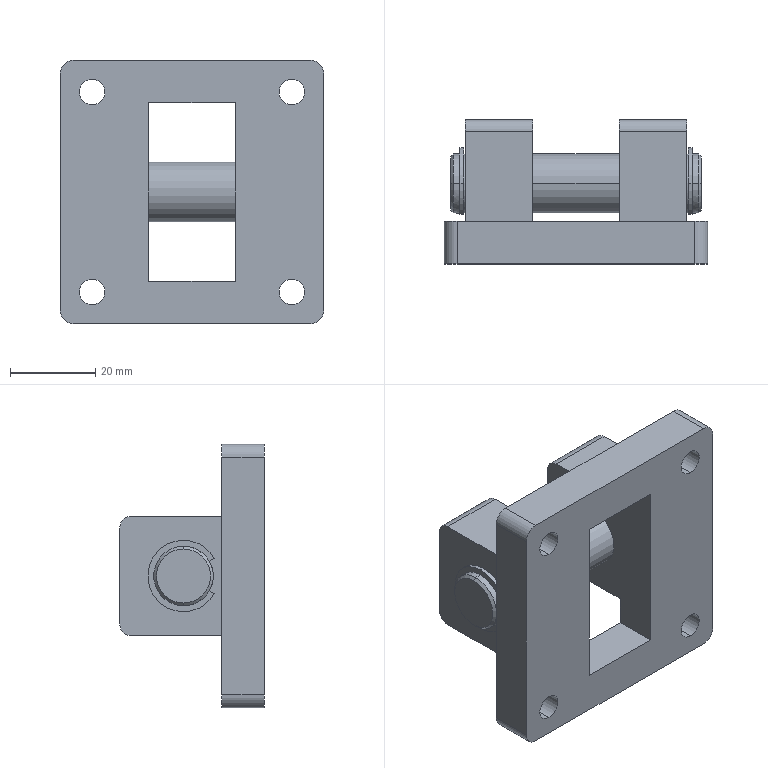Part | STEP file | 1 solid | 70 faces | box 62 x 34 x 62 mm | volume 54328 mm3 | cylinder 34 | plane 32 | cone 4 | commonest cylinder face diameters 14 x10 6 x8 16.8 x6 5.64 x4 6.2 x4 12.6 x2